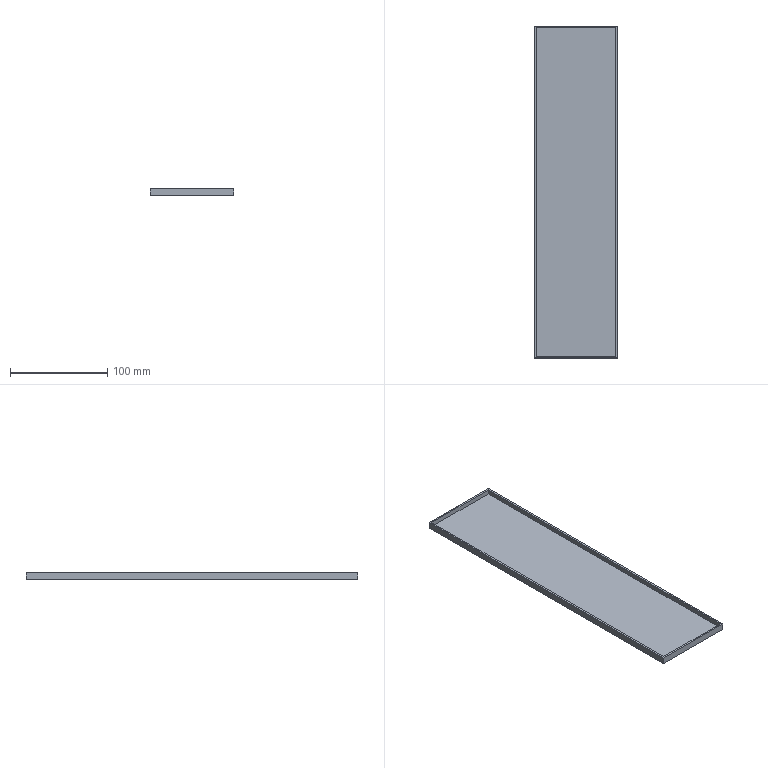Part | NX | features solid 2 | 1 solid | 11 faces | box 86 x 341 x 7 mm | volume 67112 mm3 | plane 11
STEP:
#1=CARTESIAN_POINT('',(82.,-503.,-283.));
#2=VERTEX_POINT('',#1);
#3=CARTESIAN_POINT('',(168.,-503.,-283.));
#4=VERTEX_POINT('',#3);
#5=CARTESIAN_POINT('',(330.,-503.,-283.));
#6=DIRECTION('',(1.,0.,0.));
#7=VECTOR('',#6,1000.);
#8=LINE('',#5,#7);
#9=EDGE_CURVE('',#2,#4,#8,.T.);
#10=ORIENTED_EDGE('',*,*,#9,.T.);
#11=CARTESIAN_POINT('',(168.,-162.,-283.));
#12=VERTEX_POINT('',#11);
#13=CARTESIAN_POINT('',(168.,-510.,-283.));
#14=DIRECTION('',(0.,1.,0.));
#15=VECTOR('',#14,1000.);
#16=LINE('',#13,#15);
#17=EDGE_CURVE('',#4,#12,#16,.T.);
#18=ORIENTED_EDGE('',*,*,#17,.T.);
#19=CARTESIAN_POINT('',(82.,-162.,-283.));
#20=VERTEX_POINT('',#19);
#21=CARTESIAN_POINT('',(165.,-162.,-283.));
#22=DIRECTION('',(-1.,0.,0.));
#23=VECTOR('',#22,1000.);
#24=LINE('',#21,#23);
#25=EDGE_CURVE('',#12,#20,#24,.T.);
#26=ORIENTED_EDGE('',*,*,#25,.T.);
#27=CARTESIAN_POINT('',(82.,-165.,-283.));
#28=DIRECTION('',(0.,-1.,0.));
#29=VECTOR('',#28,1000.);
#30=LINE('',#27,#29);
#31=EDGE_CURVE('',#20,#2,#30,.T.);
#32=ORIENTED_EDGE('',*,*,#31,.T.);
#33=EDGE_LOOP('',(#10,#18,#26,#32));
#34=FACE_BOUND('',#33,.T.);
#35=CARTESIAN_POINT('',(84.,-501.,-283.));
#36=VERTEX_POINT('',#35);
#37=CARTESIAN_POINT('',(166.,-501.,-283.));
#38=VERTEX_POINT('',#37);
#39=CARTESIAN_POINT('',(330.,-501.,-283.));
#40=DIRECTION('',(1.,0.,0.));
#41=VECTOR('',#40,1000.);
#42=LINE('',#39,#41);
#43=EDGE_CURVE('',#36,#38,#42,.T.);
#44=ORIENTED_EDGE('',*,*,#43,.F.);
#45=CARTESIAN_POINT('',(84.,-164.,-283.));
#46=VERTEX_POINT('',#45);
#47=CARTESIAN_POINT('',(84.,-165.,-283.));
#48=DIRECTION('',(0.,-1.,0.));
#49=VECTOR('',#48,1000.);
#50=LINE('',#47,#49);
#51=EDGE_CURVE('',#46,#36,#50,.T.);
#52=ORIENTED_EDGE('',*,*,#51,.F.);
#53=CARTESIAN_POINT('',(166.,-164.,-283.));
#54=VERTEX_POINT('',#53);
#55=CARTESIAN_POINT('',(165.,-164.,-283.));
#56=DIRECTION('',(-1.,0.,0.));
#57=VECTOR('',#56,1000.);
#58=LINE('',#55,#57);
#59=EDGE_CURVE('',#54,#46,#58,.T.);
#60=ORIENTED_EDGE('',*,*,#59,.F.);
#61=CARTESIAN_POINT('',(166.,-510.,-283.));
#62=DIRECTION('',(0.,1.,0.));
#63=VECTOR('',#62,1000.);
#64=LINE('',#61,#63);
#65=EDGE_CURVE('',#38,#54,#64,.T.);
#66=ORIENTED_EDGE('',*,*,#65,.F.);
#67=EDGE_LOOP('',(#44,#52,#60,#66));
#68=FACE_BOUND('',#67,.T.);
#69=CARTESIAN_POINT('',(165.,-510.,-283.));
#70=DIRECTION('',(0.,0.,-1.));
#71=DIRECTION('',(1.,0.,0.));
#72=AXIS2_PLACEMENT_3D('',#69,#70,#71);
#73=PLANE('',#72);
#74=ADVANCED_FACE('',(#34,#68),#73,.F.);
#75=ORIENTED_EDGE('',*,*,#9,.F.);
#76=CARTESIAN_POINT('',(82.,-503.,-290.));
#77=VERTEX_POINT('',#76);
#78=CARTESIAN_POINT('',(82.,-503.,-290.));
#79=DIRECTION('',(0.,0.,1.));
#80=VECTOR('',#79,1000.);
#81=LINE('',#78,#80);
#82=EDGE_CURVE('',#77,#2,#81,.T.);
#83=ORIENTED_EDGE('',*,*,#82,.F.);
#84=CARTESIAN_POINT('',(168.,-503.,-290.));
#85=VERTEX_POINT('',#84);
#86=CARTESIAN_POINT('',(330.,-503.,-290.));
#87=DIRECTION('',(1.,0.,0.));
#88=VECTOR('',#87,1000.);
#89=LINE('',#86,#88);
#90=EDGE_CURVE('',#77,#85,#89,.T.);
#91=ORIENTED_EDGE('',*,*,#90,.T.);
#92=CARTESIAN_POINT('',(168.,-503.,-290.));
#93=DIRECTION('',(0.,0.,1.));
#94=VECTOR('',#93,1000.);
#95=LINE('',#92,#94);
#96=EDGE_CURVE('',#85,#4,#95,.T.);
#97=ORIENTED_EDGE('',*,*,#96,.T.);
#98=EDGE_LOOP('',(#75,#83,#91,#97));
#99=FACE_BOUND('',#98,.T.);
#100=CARTESIAN_POINT('',(330.,-503.,-290.));
#101=DIRECTION('',(0.,-1.,0.));
#102=DIRECTION('',(1.,0.,0.));
#103=AXIS2_PLACEMENT_3D('',#100,#101,#102);
#104=PLANE('',#103);
#105=ADVANCED_FACE('',(#99),#104,.T.);
#106=ORIENTED_EDGE('',*,*,#31,.F.);
#107=CARTESIAN_POINT('',(82.,-162.,-290.));
#108=VERTEX_POINT('',#107);
#109=CARTESIAN_POINT('',(82.,-162.,-290.));
#110=DIRECTION('',(0.,0.,1.));
#111=VECTOR('',#110,1000.);
#112=LINE('',#109,#111);
#113=EDGE_CURVE('',#108,#20,#112,.T.);
#114=ORIENTED_EDGE('',*,*,#113,.F.);
#115=CARTESIAN_POINT('',(82.,-165.,-290.));
#116=DIRECTION('',(0.,-1.,0.));
#117=VECTOR('',#116,1000.);
#118=LINE('',#115,#117);
#119=EDGE_CURVE('',#108,#77,#118,.T.);
#120=ORIENTED_EDGE('',*,*,#119,.T.);
#121=ORIENTED_EDGE('',*,*,#82,.T.);
#122=EDGE_LOOP('',(#106,#114,#120,#121));
#123=FACE_BOUND('',#122,.T.);
#124=CARTESIAN_POINT('',(82.,-165.,-290.));
#125=DIRECTION('',(-1.,0.,0.));
#126=DIRECTION('',(0.,0.,1.));
#127=AXIS2_PLACEMENT_3D('',#124,#125,#126);
#128=PLANE('',#127);
#129=ADVANCED_FACE('',(#123),#128,.T.);
#130=ORIENTED_EDGE('',*,*,#25,.F.);
#131=CARTESIAN_POINT('',(168.,-162.,-290.));
#132=VERTEX_POINT('',#131);
#133=CARTESIAN_POINT('',(168.,-162.,-290.));
#134=DIRECTION('',(0.,0.,1.));
#135=VECTOR('',#134,1000.);
#136=LINE('',#133,#135);
#137=EDGE_CURVE('',#132,#12,#136,.T.);
#138=ORIENTED_EDGE('',*,*,#137,.F.);
#139=CARTESIAN_POINT('',(165.,-162.,-290.));
#140=DIRECTION('',(-1.,0.,0.));
#141=VECTOR('',#140,1000.);
#142=LINE('',#139,#141);
#143=EDGE_CURVE('',#132,#108,#142,.T.);
#144=ORIENTED_EDGE('',*,*,#143,.T.);
#145=ORIENTED_EDGE('',*,*,#113,.T.);
#146=EDGE_LOOP('',(#130,#138,#144,#145));
#147=FACE_BOUND('',#146,.T.);
#148=CARTESIAN_POINT('',(165.,-162.,-290.));
#149=DIRECTION('',(0.,1.,0.));
#150=DIRECTION('',(0.,0.,1.));
#151=AXIS2_PLACEMENT_3D('',#148,#149,#150);
#152=PLANE('',#151);
#153=ADVANCED_FACE('',(#147),#152,.T.);
#154=ORIENTED_EDGE('',*,*,#17,.F.);
#155=ORIENTED_EDGE('',*,*,#96,.F.);
#156=CARTESIAN_POINT('',(168.,-510.,-290.));
#157=DIRECTION('',(0.,1.,0.));
#158=VECTOR('',#157,1000.);
#159=LINE('',#156,#158);
#160=EDGE_CURVE('',#85,#132,#159,.T.);
#161=ORIENTED_EDGE('',*,*,#160,.T.);
#162=ORIENTED_EDGE('',*,*,#137,.T.);
#163=EDGE_LOOP('',(#154,#155,#161,#162));
#164=FACE_BOUND('',#163,.T.);
#165=CARTESIAN_POINT('',(168.,-510.,-290.));
#166=DIRECTION('',(1.,0.,0.));
#167=DIRECTION('',(0.,0.,-1.));
#168=AXIS2_PLACEMENT_3D('',#165,#166,#167);
#169=PLANE('',#168);
#170=ADVANCED_FACE('',(#164),#169,.T.);
#171=ORIENTED_EDGE('',*,*,#90,.F.);
#172=ORIENTED_EDGE('',*,*,#119,.F.);
#173=ORIENTED_EDGE('',*,*,#143,.F.);
#174=ORIENTED_EDGE('',*,*,#160,.F.);
#175=EDGE_LOOP('',(#171,#172,#173,#174));
#176=FACE_BOUND('',#175,.T.);
#177=CARTESIAN_POINT('',(165.,-510.,-290.));
#178=DIRECTION('',(0.,0.,-1.));
#179=DIRECTION('',(1.,0.,0.));
#180=AXIS2_PLACEMENT_3D('',#177,#178,#179);
#181=PLANE('',#180);
#182=ADVANCED_FACE('',(#176),#181,.T.);
#183=ORIENTED_EDGE('',*,*,#43,.T.);
#184=CARTESIAN_POINT('',(166.,-501.,-288.));
#185=VERTEX_POINT('',#184);
#186=CARTESIAN_POINT('',(166.,-501.,-290.));
#187=DIRECTION('',(0.,0.,1.));
#188=VECTOR('',#187,1000.);
#189=LINE('',#186,#188);
#190=EDGE_CURVE('',#185,#38,#189,.T.);
#191=ORIENTED_EDGE('',*,*,#190,.F.);
#192=CARTESIAN_POINT('',(84.,-501.,-288.));
#193=VERTEX_POINT('',#192);
#194=CARTESIAN_POINT('',(330.,-501.,-288.));
#195=DIRECTION('',(1.,0.,0.));
#196=VECTOR('',#195,1000.);
#197=LINE('',#194,#196);
#198=EDGE_CURVE('',#193,#185,#197,.T.);
#199=ORIENTED_EDGE('',*,*,#198,.F.);
#200=CARTESIAN_POINT('',(84.,-501.,-290.));
#201=DIRECTION('',(0.,0.,1.));
#202=VECTOR('',#201,1000.);
#203=LINE('',#200,#202);
#204=EDGE_CURVE('',#193,#36,#203,.T.);
#205=ORIENTED_EDGE('',*,*,#204,.T.);
#206=EDGE_LOOP('',(#183,#191,#199,#205));
#207=FACE_BOUND('',#206,.T.);
#208=CARTESIAN_POINT('',(330.,-501.,-290.));
#209=DIRECTION('',(0.,-1.,0.));
#210=DIRECTION('',(1.,0.,0.));
#211=AXIS2_PLACEMENT_3D('',#208,#209,#210);
#212=PLANE('',#211);
#213=ADVANCED_FACE('',(#207),#212,.F.);
#214=ORIENTED_EDGE('',*,*,#51,.T.);
#215=ORIENTED_EDGE('',*,*,#204,.F.);
#216=CARTESIAN_POINT('',(84.,-164.,-288.));
#217=VERTEX_POINT('',#216);
#218=CARTESIAN_POINT('',(84.,-165.,-288.));
#219=DIRECTION('',(0.,-1.,0.));
#220=VECTOR('',#219,1000.);
#221=LINE('',#218,#220);
#222=EDGE_CURVE('',#217,#193,#221,.T.);
#223=ORIENTED_EDGE('',*,*,#222,.F.);
#224=CARTESIAN_POINT('',(84.,-164.,-290.));
#225=DIRECTION('',(0.,0.,1.));
#226=VECTOR('',#225,1000.);
#227=LINE('',#224,#226);
#228=EDGE_CURVE('',#217,#46,#227,.T.);
#229=ORIENTED_EDGE('',*,*,#228,.T.);
#230=EDGE_LOOP('',(#214,#215,#223,#229));
#231=FACE_BOUND('',#230,.T.);
#232=CARTESIAN_POINT('',(84.,-165.,-290.));
#233=DIRECTION('',(-1.,0.,0.));
#234=DIRECTION('',(0.,0.,1.));
#235=AXIS2_PLACEMENT_3D('',#232,#233,#234);
#236=PLANE('',#235);
#237=ADVANCED_FACE('',(#231),#236,.F.);
#238=ORIENTED_EDGE('',*,*,#59,.T.);
#239=ORIENTED_EDGE('',*,*,#228,.F.);
#240=CARTESIAN_POINT('',(166.,-164.,-288.));
#241=VERTEX_POINT('',#240);
#242=CARTESIAN_POINT('',(165.,-164.,-288.));
#243=DIRECTION('',(-1.,0.,0.));
#244=VECTOR('',#243,1000.);
#245=LINE('',#242,#244);
#246=EDGE_CURVE('',#241,#217,#245,.T.);
#247=ORIENTED_EDGE('',*,*,#246,.F.);
#248=CARTESIAN_POINT('',(166.,-164.,-290.));
#249=DIRECTION('',(0.,0.,1.));
#250=VECTOR('',#249,1000.);
#251=LINE('',#248,#250);
#252=EDGE_CURVE('',#241,#54,#251,.T.);
#253=ORIENTED_EDGE('',*,*,#252,.T.);
#254=EDGE_LOOP('',(#238,#239,#247,#253));
#255=FACE_BOUND('',#254,.T.);
#256=CARTESIAN_POINT('',(165.,-164.,-290.));
#257=DIRECTION('',(0.,1.,0.));
#258=DIRECTION('',(0.,0.,1.));
#259=AXIS2_PLACEMENT_3D('',#256,#257,#258);
#260=PLANE('',#259);
#261=ADVANCED_FACE('',(#255),#260,.F.);
#262=ORIENTED_EDGE('',*,*,#65,.T.);
#263=ORIENTED_EDGE('',*,*,#252,.F.);
#264=CARTESIAN_POINT('',(166.,-510.,-288.));
#265=DIRECTION('',(0.,1.,0.));
#266=VECTOR('',#265,1000.);
#267=LINE('',#264,#266);
#268=EDGE_CURVE('',#185,#241,#267,.T.);
#269=ORIENTED_EDGE('',*,*,#268,.F.);
#270=ORIENTED_EDGE('',*,*,#190,.T.);
#271=EDGE_LOOP('',(#262,#263,#269,#270));
#272=FACE_BOUND('',#271,.T.);
#273=CARTESIAN_POINT('',(166.,-510.,-290.));
#274=DIRECTION('',(1.,0.,0.));
#275=DIRECTION('',(0.,0.,-1.));
#276=AXIS2_PLACEMENT_3D('',#273,#274,#275);
#277=PLANE('',#276);
#278=ADVANCED_FACE('',(#272),#277,.F.);
#279=ORIENTED_EDGE('',*,*,#198,.T.);
#280=ORIENTED_EDGE('',*,*,#268,.T.);
#281=ORIENTED_EDGE('',*,*,#246,.T.);
#282=ORIENTED_EDGE('',*,*,#222,.T.);
#283=EDGE_LOOP('',(#279,#280,#281,#282));
#284=FACE_BOUND('',#283,.T.);
#285=CARTESIAN_POINT('',(165.,-510.,-288.));
#286=DIRECTION('',(0.,0.,-1.));
#287=DIRECTION('',(1.,0.,0.));
#288=AXIS2_PLACEMENT_3D('',#285,#286,#287);
#289=PLANE('',#288);
#290=ADVANCED_FACE('',(#284),#289,.F.);
#291=CLOSED_SHELL('',(#74,#105,#129,#153,#170,#182,#213,#237,#261,#278,#290));
#292=MANIFOLD_SOLID_BREP('',#291);
#293=(LENGTH_UNIT()NAMED_UNIT(*)SI_UNIT(.MILLI.,.METRE.));
#294=UNCERTAINTY_MEASURE_WITH_UNIT(LENGTH_MEASURE(0.00001),#293,'','');
#295=(NAMED_UNIT(*)PLANE_ANGLE_UNIT()SI_UNIT($,.RADIAN.));
#296=(NAMED_UNIT(*)SI_UNIT($,.STERADIAN.)SOLID_ANGLE_UNIT());
#297=(GEOMETRIC_REPRESENTATION_CONTEXT(3)GLOBAL_UNCERTAINTY_ASSIGNED_CONTEXT((#294))GLOBAL_UNIT_ASSIGNED_CONTEXT((#293,#295,#296))REPRESENTATION_CONTEXT('',''));
#298=ADVANCED_BREP_SHAPE_REPRESENTATION('',(#292),#297);